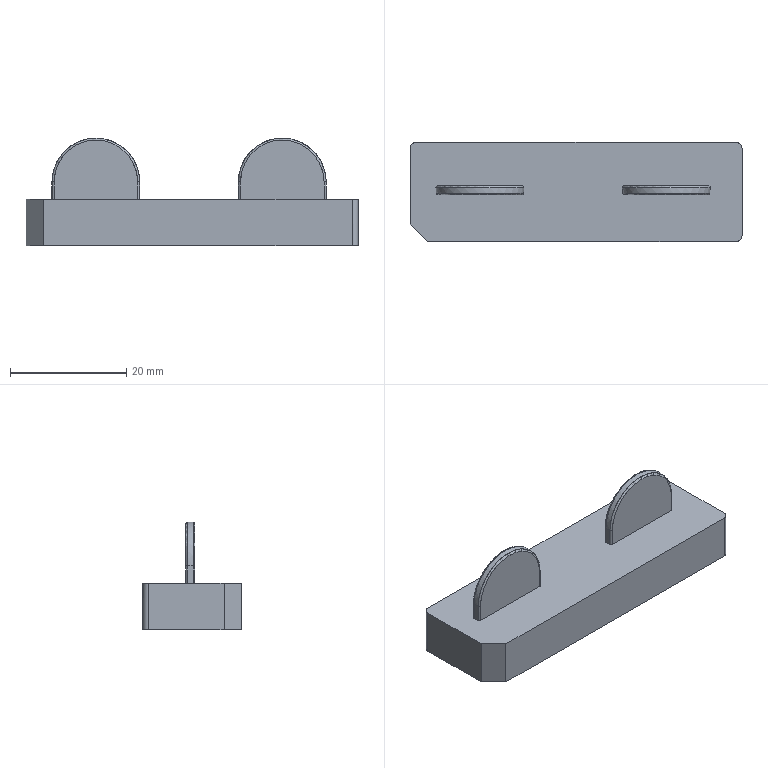CAM job | PowerMill | 3-axis milling, other | part box 57 x 17 x 18.538 mm
Tools:
number,name,type,diameter,tip_radius,length,cutting_length,overhang,flutes,holder,toolpaths_using
1,D10C,end_mill,10.0,0.0,60.0,,30.0,1,D42L35,1
1,D10C_1_1_1,end_mill,10.0,0.0,60.0,,19.0,1,D42L35,3
2,D4C_1_1,end_mill,4.0,0.0,30.0,,10.72,1,D42L35,1
3,D10_1_1_1,end_mill,10.0,0.0,60.0,,18.68,1,D42L35,3
22,R1.5_1_1,ball_nosed,3.0,1.5,30.0,,9.36,1,D42L35,1
10,D3_1_1,end_mill,3.0,0.0,30.0,,10.8,1,D42L35,1
13,Text_D4_1_1,taper_spherical,4.0,0.3,60.0,,10.8,1,D42L35,1
Operations:
program,toolpath,strategy,tool,tool_number,tool_diameter,tip_radius,flutes,spindle_rpm,feed_cut,surface_speed_m_min_computed,feed_per_tooth_computed,tolerance,thickness,stepover,stepdown,cut_length,cut_time_min,total_time_min,workplane
18-S-3-F,精公开粗01-扫面平行-D10C,raster_area_clear,D10C_1_1_1,1,10.0,0.0,1.0,8000.0,10000.0,251.33,1.25,0.03,0.28,6.0,1.0,335.36,0.034,0.0395,
18-S-3-F,精公开粗01-外形偏置-D10C,offset_area_clear,D10C_1_1_1,1,10.0,0.0,1.0,8000.0,10000.0,251.33,1.25,0.03,0.28,6.0,1.0,8777.247,0.878,0.9465,
18-S-3-F,精公开粗01-基准台等高-D10C,constantz,D10C_1_1_1,1,10.0,0.0,1.0,8000.0,10000.0,251.33,1.25,0.03,0.07,5.0,0.4,3889.063,0.389,0.3995,
18-S-3-F,精公再粗02-外形偏置-D4C,offset_area_clear,D4C_1_1,2,4.0,0.0,1.0,18000.0,6000.0,226.19,0.3333,0.03,0.0,2.0,1.0,4951.36,0.825,0.8812,
18-S-3-F,精公基准台01-基准面偏置-D10,offset_area_clear,D10_1_1_1,3,10.0,0.0,1.0,8500.0,600.0,267.04,0.0706,0.005,0.38,5.0,1.0,191.595,0.319,0.3614,
18-S-3-F,精公基准台01-外形侧光-D10,profile_area_clear,D10_1_1_1,3,10.0,0.0,1.0,8500.0,600.0,267.04,0.0706,0.005,-0.07,0.08,1.0,255.191,0.425,0.4657,
18-S-3-F,精公基准台01-基准台侧光-D10,profile_area_clear,D10_1_1_1,3,10.0,0.0,1.0,8500.0,600.0,267.04,0.0706,0.005,0.0,0.08,1.0,353.233,0.589,0.6538,
18-S-3-F,精公精光01-浅滩和陡峭-R1.5,inter_constz,R1.5_1_1,22,3.0,1.5,1.0,22000.0,2000.0,207.35,0.0909,0.005,-0.075,0.04,1.0,7694.779,3.847,4.293,
18-S-3-F,精公精光02-等高-D3,constantz,D3_1_1,10,3.0,0.0,1.0,18000.0,2000.0,169.65,0.1111,0.005,-0.075,5.0,0.03,25974.152,12.987,13.005,
18-S-3-F,精公刻字01-刻字-Text_D4,pattern,Text_D4_1_1,13,4.0,0.3,1.0,15000.0,1000.0,188.5,0.0667,0.005,0.0,5.0,1.0,91.102,0.091,0.1106,
,精公开粗01-外形偏置-D10C_Reference,offset_area_clear,D10C,1,10.0,0.0,1.0,8000.0,10000.0,251.33,1.25,0.03,0.28,6.0,1.0,17276.781,1.728,1.86,